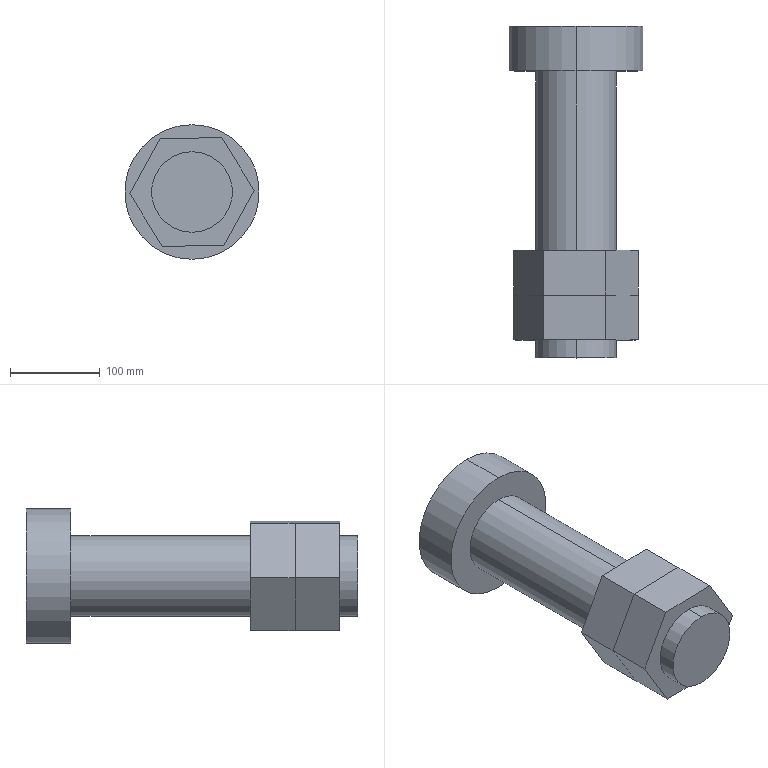Part | SolidWorks | features ICE 1, LPattern 1, Revolution 1 | 3 solids | 27 faces | box 150 x 370 x 150 mm | volume 3530229 mm3 | plane 19 | cylinder 8 | commonest cylinder face diameters 90 x6 150 x2
STEP:
#1=CARTESIAN_POINT('',(0.,345.893,-45.));
#2=VERTEX_POINT('',#1);
#3=CARTESIAN_POINT('',(0.,345.893,45.));
#4=VERTEX_POINT('',#3);
#5=CARTESIAN_POINT('',(0.,345.893,0.));
#6=DIRECTION('',(0.,-1.,0.));
#7=DIRECTION('',(0.,0.,-1.));
#8=AXIS2_PLACEMENT_3D('',#5,#6,#7);
#9=CIRCLE('',#8,45.);
#10=EDGE_CURVE('',#2,#4,#9,.T.);
#11=ORIENTED_EDGE('',*,*,#10,.T.);
#12=CARTESIAN_POINT('',(0.,25.893,45.));
#13=VERTEX_POINT('',#12);
#14=CARTESIAN_POINT('',(0.,0.,45.));
#15=DIRECTION('',(0.,-1.,0.));
#16=VECTOR('',#15,1000.);
#17=LINE('',#14,#16);
#18=EDGE_CURVE('',#4,#13,#17,.T.);
#19=ORIENTED_EDGE('',*,*,#18,.T.);
#20=CARTESIAN_POINT('',(0.,25.893,-45.));
#21=VERTEX_POINT('',#20);
#22=CARTESIAN_POINT('',(0.,25.893,0.));
#23=DIRECTION('',(0.,-1.,0.));
#24=DIRECTION('',(0.,0.,-1.));
#25=AXIS2_PLACEMENT_3D('',#22,#23,#24);
#26=CIRCLE('',#25,45.);
#27=EDGE_CURVE('',#21,#13,#26,.T.);
#28=ORIENTED_EDGE('',*,*,#27,.F.);
#29=CARTESIAN_POINT('',(0.,0.,-45.));
#30=DIRECTION('',(0.,-1.,0.));
#31=VECTOR('',#30,1000.);
#32=LINE('',#29,#31);
#33=EDGE_CURVE('',#2,#21,#32,.T.);
#34=ORIENTED_EDGE('',*,*,#33,.F.);
#35=EDGE_LOOP('',(#11,#19,#28,#34));
#36=FACE_OUTER_BOUND('',#35,.T.);
#37=CARTESIAN_POINT('',(0.,0.,0.));
#38=DIRECTION('',(0.,-1.,0.));
#39=DIRECTION('',(0.,0.,-1.));
#40=AXIS2_PLACEMENT_3D('',#37,#38,#39);
#41=CYLINDRICAL_SURFACE('',#40,45.);
#42=ADVANCED_FACE('',(#36),#41,.T.);
#43=CARTESIAN_POINT('',(0.,395.893,-75.));
#44=VERTEX_POINT('',#43);
#45=CARTESIAN_POINT('',(0.,395.893,75.));
#46=VERTEX_POINT('',#45);
#47=CARTESIAN_POINT('',(0.,395.893,0.));
#48=DIRECTION('',(0.,-1.,0.));
#49=DIRECTION('',(0.,0.,-1.));
#50=AXIS2_PLACEMENT_3D('',#47,#48,#49);
#51=CIRCLE('',#50,75.);
#52=EDGE_CURVE('',#44,#46,#51,.T.);
#53=ORIENTED_EDGE('',*,*,#52,.T.);
#54=CARTESIAN_POINT('',(0.,345.893,75.));
#55=VERTEX_POINT('',#54);
#56=CARTESIAN_POINT('',(0.,0.,75.));
#57=DIRECTION('',(0.,-1.,0.));
#58=VECTOR('',#57,1000.);
#59=LINE('',#56,#58);
#60=EDGE_CURVE('',#46,#55,#59,.T.);
#61=ORIENTED_EDGE('',*,*,#60,.T.);
#62=CARTESIAN_POINT('',(0.,345.893,-75.));
#63=VERTEX_POINT('',#62);
#64=CARTESIAN_POINT('',(0.,345.893,0.));
#65=DIRECTION('',(0.,-1.,0.));
#66=DIRECTION('',(0.,0.,-1.));
#67=AXIS2_PLACEMENT_3D('',#64,#65,#66);
#68=CIRCLE('',#67,75.);
#69=EDGE_CURVE('',#63,#55,#68,.T.);
#70=ORIENTED_EDGE('',*,*,#69,.F.);
#71=CARTESIAN_POINT('',(0.,0.,-75.));
#72=DIRECTION('',(0.,-1.,0.));
#73=VECTOR('',#72,1000.);
#74=LINE('',#71,#73);
#75=EDGE_CURVE('',#44,#63,#74,.T.);
#76=ORIENTED_EDGE('',*,*,#75,.F.);
#77=EDGE_LOOP('',(#53,#61,#70,#76));
#78=FACE_OUTER_BOUND('',#77,.T.);
#79=CARTESIAN_POINT('',(0.,0.,0.));
#80=DIRECTION('',(0.,-1.,0.));
#81=DIRECTION('',(0.,0.,-1.));
#82=AXIS2_PLACEMENT_3D('',#79,#80,#81);
#83=CYLINDRICAL_SURFACE('',#82,75.);
#84=ADVANCED_FACE('',(#78),#83,.T.);
#85=ORIENTED_EDGE('',*,*,#52,.F.);
#86=CARTESIAN_POINT('',(0.,395.893,0.));
#87=DIRECTION('',(0.,-1.,0.));
#88=DIRECTION('',(0.,0.,-1.));
#89=AXIS2_PLACEMENT_3D('',#86,#87,#88);
#90=CIRCLE('',#89,75.);
#91=EDGE_CURVE('',#46,#44,#90,.T.);
#92=ORIENTED_EDGE('',*,*,#91,.F.);
#93=EDGE_LOOP('',(#85,#92));
#94=FACE_OUTER_BOUND('',#93,.T.);
#95=CARTESIAN_POINT('',(0.,395.893,0.));
#96=DIRECTION('',(0.,1.,0.));
#97=DIRECTION('',(0.,0.,1.));
#98=AXIS2_PLACEMENT_3D('',#95,#96,#97);
#99=PLANE('',#98);
#100=ADVANCED_FACE('',(#94),#99,.T.);
#101=ORIENTED_EDGE('',*,*,#60,.F.);
#102=ORIENTED_EDGE('',*,*,#91,.T.);
#103=ORIENTED_EDGE('',*,*,#75,.T.);
#104=CARTESIAN_POINT('',(0.,345.893,0.));
#105=DIRECTION('',(0.,-1.,0.));
#106=DIRECTION('',(0.,0.,-1.));
#107=AXIS2_PLACEMENT_3D('',#104,#105,#106);
#108=CIRCLE('',#107,75.);
#109=EDGE_CURVE('',#55,#63,#108,.T.);
#110=ORIENTED_EDGE('',*,*,#109,.F.);
#111=EDGE_LOOP('',(#101,#102,#103,#110));
#112=FACE_OUTER_BOUND('',#111,.T.);
#113=CARTESIAN_POINT('',(0.,0.,0.));
#114=DIRECTION('',(0.,-1.,0.));
#115=DIRECTION('',(0.,0.,-1.));
#116=AXIS2_PLACEMENT_3D('',#113,#114,#115);
#117=CYLINDRICAL_SURFACE('',#116,75.);
#118=ADVANCED_FACE('',(#112),#117,.T.);
#119=ORIENTED_EDGE('',*,*,#69,.T.);
#120=ORIENTED_EDGE('',*,*,#109,.T.);
#121=EDGE_LOOP('',(#119,#120));
#122=FACE_OUTER_BOUND('',#121,.T.);
#123=ORIENTED_EDGE('',*,*,#10,.F.);
#124=CARTESIAN_POINT('',(0.,345.893,0.));
#125=DIRECTION('',(0.,-1.,0.));
#126=DIRECTION('',(0.,0.,-1.));
#127=AXIS2_PLACEMENT_3D('',#124,#125,#126);
#128=CIRCLE('',#127,45.);
#129=EDGE_CURVE('',#4,#2,#128,.T.);
#130=ORIENTED_EDGE('',*,*,#129,.F.);
#131=EDGE_LOOP('',(#123,#130));
#132=FACE_BOUND('',#131,.T.);
#133=CARTESIAN_POINT('',(75.,345.893,0.));
#134=DIRECTION('',(0.,-1.,0.));
#135=DIRECTION('',(0.,0.,-1.));
#136=AXIS2_PLACEMENT_3D('',#133,#134,#135);
#137=PLANE('',#136);
#138=ADVANCED_FACE('',(#122,#132),#137,.T.);
#139=ORIENTED_EDGE('',*,*,#18,.F.);
#140=ORIENTED_EDGE('',*,*,#129,.T.);
#141=ORIENTED_EDGE('',*,*,#33,.T.);
#142=CARTESIAN_POINT('',(0.,25.893,0.));
#143=DIRECTION('',(0.,-1.,0.));
#144=DIRECTION('',(0.,0.,-1.));
#145=AXIS2_PLACEMENT_3D('',#142,#143,#144);
#146=CIRCLE('',#145,45.);
#147=EDGE_CURVE('',#13,#21,#146,.T.);
#148=ORIENTED_EDGE('',*,*,#147,.F.);
#149=EDGE_LOOP('',(#139,#140,#141,#148));
#150=FACE_OUTER_BOUND('',#149,.T.);
#151=CARTESIAN_POINT('',(0.,0.,0.));
#152=DIRECTION('',(0.,-1.,0.));
#153=DIRECTION('',(0.,0.,-1.));
#154=AXIS2_PLACEMENT_3D('',#151,#152,#153);
#155=CYLINDRICAL_SURFACE('',#154,45.);
#156=ADVANCED_FACE('',(#150),#155,.T.);
#157=ORIENTED_EDGE('',*,*,#27,.T.);
#158=ORIENTED_EDGE('',*,*,#147,.T.);
#159=EDGE_LOOP('',(#157,#158));
#160=FACE_OUTER_BOUND('',#159,.T.);
#161=CARTESIAN_POINT('',(45.,25.893,0.));
#162=DIRECTION('',(0.,-1.,0.));
#163=DIRECTION('',(0.,0.,-1.));
#164=AXIS2_PLACEMENT_3D('',#161,#162,#163);
#165=PLANE('',#164);
#166=ADVANCED_FACE('',(#160),#165,.T.);
#167=CLOSED_SHELL('',(#42,#84,#100,#118,#138,#156,#166));
#168=MANIFOLD_SOLID_BREP('',#167);
#169=CARTESIAN_POINT('',(0.,95.893,45.));
#170=VERTEX_POINT('',#169);
#171=CARTESIAN_POINT('',(0.,95.893,-45.));
#172=VERTEX_POINT('',#171);
#173=CARTESIAN_POINT('',(0.,95.893,0.));
#174=DIRECTION('',(0.,-1.,0.));
#175=DIRECTION('',(0.,0.,-1.));
#176=AXIS2_PLACEMENT_3D('',#173,#174,#175);
#177=CIRCLE('',#176,45.);
#178=EDGE_CURVE('',#170,#172,#177,.T.);
#179=ORIENTED_EDGE('',*,*,#178,.T.);
#180=CARTESIAN_POINT('',(0.,145.893,-45.));
#181=VERTEX_POINT('',#180);
#182=CARTESIAN_POINT('',(0.,95.893,-45.));
#183=DIRECTION('',(0.,1.,0.));
#184=VECTOR('',#183,1000.);
#185=LINE('',#182,#184);
#186=EDGE_CURVE('',#172,#181,#185,.T.);
#187=ORIENTED_EDGE('',*,*,#186,.T.);
#188=CARTESIAN_POINT('',(0.,145.893,45.));
#189=VERTEX_POINT('',#188);
#190=CARTESIAN_POINT('',(0.,145.893,0.));
#191=DIRECTION('',(0.,-1.,0.));
#192=DIRECTION('',(0.,0.,-1.));
#193=AXIS2_PLACEMENT_3D('',#190,#191,#192);
#194=CIRCLE('',#193,45.);
#195=EDGE_CURVE('',#189,#181,#194,.T.);
#196=ORIENTED_EDGE('',*,*,#195,.F.);
#197=CARTESIAN_POINT('',(0.,95.893,45.));
#198=DIRECTION('',(0.,1.,0.));
#199=VECTOR('',#198,1000.);
#200=LINE('',#197,#199);
#201=EDGE_CURVE('',#170,#189,#200,.T.);
#202=ORIENTED_EDGE('',*,*,#201,.F.);
#203=EDGE_LOOP('',(#179,#187,#196,#202));
#204=FACE_OUTER_BOUND('',#203,.T.);
#205=CARTESIAN_POINT('',(0.,95.893,0.));
#206=DIRECTION('',(0.,1.,0.));
#207=DIRECTION('',(0.,0.,1.));
#208=AXIS2_PLACEMENT_3D('',#205,#206,#207);
#209=CYLINDRICAL_SURFACE('',#208,45.);
#210=ADVANCED_FACE('',(#204),#209,.F.);
#211=CARTESIAN_POINT('',(69.26,95.893,1.765));
#212=VERTEX_POINT('',#211);
#213=CARTESIAN_POINT('',(33.101,95.893,60.863));
#214=VERTEX_POINT('',#213);
#215=CARTESIAN_POINT('',(69.26,95.893,1.765));
#216=DIRECTION('',(-0.5219,0.,0.853));
#217=VECTOR('',#216,1000.);
#218=LINE('',#215,#217);
#219=EDGE_CURVE('',#212,#214,#218,.T.);
#220=ORIENTED_EDGE('',*,*,#219,.T.);
#221=CARTESIAN_POINT('',(-36.159,95.893,59.098));
#222=VERTEX_POINT('',#221);
#223=CARTESIAN_POINT('',(33.101,95.893,60.863));
#224=DIRECTION('',(-0.9997,0.,-0.02548));
#225=VECTOR('',#224,1000.);
#226=LINE('',#223,#225);
#227=EDGE_CURVE('',#214,#222,#226,.T.);
#228=ORIENTED_EDGE('',*,*,#227,.T.);
#229=CARTESIAN_POINT('',(-69.26,95.893,-1.765));
#230=VERTEX_POINT('',#229);
#231=CARTESIAN_POINT('',(-36.159,95.893,59.098));
#232=DIRECTION('',(-0.4778,0.,-0.8785));
#233=VECTOR('',#232,1000.);
#234=LINE('',#231,#233);
#235=EDGE_CURVE('',#222,#230,#234,.T.);
#236=ORIENTED_EDGE('',*,*,#235,.T.);
#237=CARTESIAN_POINT('',(-33.101,95.893,-60.863));
#238=VERTEX_POINT('',#237);
#239=CARTESIAN_POINT('',(-69.26,95.893,-1.765));
#240=DIRECTION('',(0.5219,0.,-0.853));
#241=VECTOR('',#240,1000.);
#242=LINE('',#239,#241);
#243=EDGE_CURVE('',#230,#238,#242,.T.);
#244=ORIENTED_EDGE('',*,*,#243,.T.);
#245=CARTESIAN_POINT('',(36.159,95.893,-59.098));
#246=VERTEX_POINT('',#245);
#247=CARTESIAN_POINT('',(-33.101,95.893,-60.863));
#248=DIRECTION('',(0.9997,0.,0.02548));
#249=VECTOR('',#248,1000.);
#250=LINE('',#247,#249);
#251=EDGE_CURVE('',#238,#246,#250,.T.);
#252=ORIENTED_EDGE('',*,*,#251,.T.);
#253=CARTESIAN_POINT('',(36.159,95.893,-59.098));
#254=DIRECTION('',(0.4778,0.,0.8785));
#255=VECTOR('',#254,1000.);
#256=LINE('',#253,#255);
#257=EDGE_CURVE('',#246,#212,#256,.T.);
#258=ORIENTED_EDGE('',*,*,#257,.T.);
#259=EDGE_LOOP('',(#220,#228,#236,#244,#252,#258));
#260=FACE_OUTER_BOUND('',#259,.T.);
#261=ORIENTED_EDGE('',*,*,#178,.F.);
#262=CARTESIAN_POINT('',(0.,95.893,0.));
#263=DIRECTION('',(0.,-1.,0.));
#264=DIRECTION('',(0.,0.,-1.));
#265=AXIS2_PLACEMENT_3D('',#262,#263,#264);
#266=CIRCLE('',#265,45.);
#267=EDGE_CURVE('',#172,#170,#266,.T.);
#268=ORIENTED_EDGE('',*,*,#267,.F.);
#269=EDGE_LOOP('',(#261,#268));
#270=FACE_BOUND('',#269,.T.);
#271=CARTESIAN_POINT('',(0.,95.893,0.));
#272=DIRECTION('',(0.,-1.,0.));
#273=DIRECTION('',(0.,0.,-1.));
#274=AXIS2_PLACEMENT_3D('',#271,#272,#273);
#275=PLANE('',#274);
#276=ADVANCED_FACE('',(#260,#270),#275,.T.);
#277=CARTESIAN_POINT('',(69.26,145.893,1.765));
#278=VERTEX_POINT('',#277);
#279=CARTESIAN_POINT('',(33.101,145.893,60.863));
#280=VERTEX_POINT('',#279);
#281=CARTESIAN_POINT('',(69.26,145.893,1.765));
#282=DIRECTION('',(-0.5219,0.,0.853));
#283=VECTOR('',#282,1000.);
#284=LINE('',#281,#283);
#285=EDGE_CURVE('',#278,#280,#284,.T.);
#286=ORIENTED_EDGE('',*,*,#285,.F.);
#287=CARTESIAN_POINT('',(36.159,145.893,-59.098));
#288=VERTEX_POINT('',#287);
#289=CARTESIAN_POINT('',(36.159,145.893,-59.098));
#290=DIRECTION('',(0.4778,0.,0.8785));
#291=VECTOR('',#290,1000.);
#292=LINE('',#289,#291);
#293=EDGE_CURVE('',#288,#278,#292,.T.);
#294=ORIENTED_EDGE('',*,*,#293,.F.);
#295=CARTESIAN_POINT('',(-33.101,145.893,-60.863));
#296=VERTEX_POINT('',#295);
#297=CARTESIAN_POINT('',(-33.101,145.893,-60.863));
#298=DIRECTION('',(0.9997,0.,0.02548));
#299=VECTOR('',#298,1000.);
#300=LINE('',#297,#299);
#301=EDGE_CURVE('',#296,#288,#300,.T.);
#302=ORIENTED_EDGE('',*,*,#301,.F.);
#303=CARTESIAN_POINT('',(-69.26,145.893,-1.765));
#304=VERTEX_POINT('',#303);
#305=CARTESIAN_POINT('',(-69.26,145.893,-1.765));
#306=DIRECTION('',(0.5219,0.,-0.853));
#307=VECTOR('',#306,1000.);
#308=LINE('',#305,#307);
#309=EDGE_CURVE('',#304,#296,#308,.T.);
#310=ORIENTED_EDGE('',*,*,#309,.F.);
#311=CARTESIAN_POINT('',(-36.159,145.893,59.098));
#312=VERTEX_POINT('',#311);
#313=CARTESIAN_POINT('',(-36.159,145.893,59.098));
#314=DIRECTION('',(-0.4778,0.,-0.8785));
#315=VECTOR('',#314,1000.);
#316=LINE('',#313,#315);
#317=EDGE_CURVE('',#312,#304,#316,.T.);
#318=ORIENTED_EDGE('',*,*,#317,.F.);
#319=CARTESIAN_POINT('',(33.101,145.893,60.863));
#320=DIRECTION('',(-0.9997,0.,-0.02548));
#321=VECTOR('',#320,1000.);
#322=LINE('',#319,#321);
#323=EDGE_CURVE('',#280,#312,#322,.T.);
#324=ORIENTED_EDGE('',*,*,#323,.F.);
#325=EDGE_LOOP('',(#286,#294,#302,#310,#318,#324));
#326=FACE_OUTER_BOUND('',#325,.T.);
#327=ORIENTED_EDGE('',*,*,#195,.T.);
#328=CARTESIAN_POINT('',(0.,145.893,0.));
#329=DIRECTION('',(0.,-1.,0.));
#330=DIRECTION('',(0.,0.,-1.));
#331=AXIS2_PLACEMENT_3D('',#328,#329,#330);
#332=CIRCLE('',#331,45.);
#333=EDGE_CURVE('',#181,#189,#332,.T.);
#334=ORIENTED_EDGE('',*,*,#333,.T.);
#335=EDGE_LOOP('',(#327,#334));
#336=FACE_BOUND('',#335,.T.);
#337=CARTESIAN_POINT('',(0.,145.893,0.));
#338=DIRECTION('',(0.,-1.,0.));
#339=DIRECTION('',(0.,0.,-1.));
#340=AXIS2_PLACEMENT_3D('',#337,#338,#339);
#341=PLANE('',#340);
#342=ADVANCED_FACE('',(#326,#336),#341,.F.);
#343=ORIENTED_EDGE('',*,*,#285,.T.);
#344=CARTESIAN_POINT('',(33.101,95.893,60.863));
#345=DIRECTION('',(0.,1.,0.));
#346=VECTOR('',#345,1000.);
#347=LINE('',#344,#346);
#348=EDGE_CURVE('',#214,#280,#347,.T.);
#349=ORIENTED_EDGE('',*,*,#348,.F.);
#350=ORIENTED_EDGE('',*,*,#219,.F.);
#351=CARTESIAN_POINT('',(69.26,95.893,1.765));
#352=DIRECTION('',(0.,1.,0.));
#353=VECTOR('',#352,1000.);
#354=LINE('',#351,#353);
#355=EDGE_CURVE('',#212,#278,#354,.T.);
#356=ORIENTED_EDGE('',*,*,#355,.T.);
#357=EDGE_LOOP('',(#343,#349,#350,#356));
#358=FACE_OUTER_BOUND('',#357,.T.);
#359=CARTESIAN_POINT('',(69.26,95.893,1.765));
#360=DIRECTION('',(-0.853,0.,-0.5219));
#361=DIRECTION('',(-0.5219,0.,0.853));
#362=AXIS2_PLACEMENT_3D('',#359,#360,#361);
#363=PLANE('',#362);
#364=ADVANCED_FACE('',(#358),#363,.F.);
#365=ORIENTED_EDGE('',*,*,#323,.T.);
#366=CARTESIAN_POINT('',(-36.159,95.893,59.098));
#367=DIRECTION('',(0.,1.,0.));
#368=VECTOR('',#367,1000.);
#369=LINE('',#366,#368);
#370=EDGE_CURVE('',#222,#312,#369,.T.);
#371=ORIENTED_EDGE('',*,*,#370,.F.);
#372=ORIENTED_EDGE('',*,*,#227,.F.);
#373=ORIENTED_EDGE('',*,*,#348,.T.);
#374=EDGE_LOOP('',(#365,#371,#372,#373));
#375=FACE_OUTER_BOUND('',#374,.T.);
#376=CARTESIAN_POINT('',(33.101,95.893,60.863));
#377=DIRECTION('',(0.02548,0.,-0.9997));
#378=DIRECTION('',(-0.9997,0.,-0.02548));
#379=AXIS2_PLACEMENT_3D('',#376,#377,#378);
#380=PLANE('',#379);
#381=ADVANCED_FACE('',(#375),#380,.F.);
#382=ORIENTED_EDGE('',*,*,#317,.T.);
#383=CARTESIAN_POINT('',(-69.26,95.893,-1.765));
#384=DIRECTION('',(0.,1.,0.));
#385=VECTOR('',#384,1000.);
#386=LINE('',#383,#385);
#387=EDGE_CURVE('',#230,#304,#386,.T.);
#388=ORIENTED_EDGE('',*,*,#387,.F.);
#389=ORIENTED_EDGE('',*,*,#235,.F.);
#390=ORIENTED_EDGE('',*,*,#370,.T.);
#391=EDGE_LOOP('',(#382,#388,#389,#390));
#392=FACE_OUTER_BOUND('',#391,.T.);
#393=CARTESIAN_POINT('',(-36.159,95.893,59.098));
#394=DIRECTION('',(0.8785,0.,-0.4778));
#395=DIRECTION('',(-0.4778,0.,-0.8785));
#396=AXIS2_PLACEMENT_3D('',#393,#394,#395);
#397=PLANE('',#396);
#398=ADVANCED_FACE('',(#392),#397,.F.);
#399=ORIENTED_EDGE('',*,*,#309,.T.);
#400=CARTESIAN_POINT('',(-33.101,95.893,-60.863));
#401=DIRECTION('',(0.,1.,0.));
#402=VECTOR('',#401,1000.);
#403=LINE('',#400,#402);
#404=EDGE_CURVE('',#238,#296,#403,.T.);
#405=ORIENTED_EDGE('',*,*,#404,.F.);
#406=ORIENTED_EDGE('',*,*,#243,.F.);
#407=ORIENTED_EDGE('',*,*,#387,.T.);
#408=EDGE_LOOP('',(#399,#405,#406,#407));
#409=FACE_OUTER_BOUND('',#408,.T.);
#410=CARTESIAN_POINT('',(-69.26,95.893,-1.765));
#411=DIRECTION('',(0.853,0.,0.5219));
#412=DIRECTION('',(0.5219,0.,-0.853));
#413=AXIS2_PLACEMENT_3D('',#410,#411,#412);
#414=PLANE('',#413);
#415=ADVANCED_FACE('',(#409),#414,.F.);
#416=ORIENTED_EDGE('',*,*,#301,.T.);
#417=CARTESIAN_POINT('',(36.159,95.893,-59.098));
#418=DIRECTION('',(0.,1.,0.));
#419=VECTOR('',#418,1000.);
#420=LINE('',#417,#419);
#421=EDGE_CURVE('',#246,#288,#420,.T.);
#422=ORIENTED_EDGE('',*,*,#421,.F.);
#423=ORIENTED_EDGE('',*,*,#251,.F.);
#424=ORIENTED_EDGE('',*,*,#404,.T.);
#425=EDGE_LOOP('',(#416,#422,#423,#424));
#426=FACE_OUTER_BOUND('',#425,.T.);
#427=CARTESIAN_POINT('',(-33.101,95.893,-60.863));
#428=DIRECTION('',(-0.02548,0.,0.9997));
#429=DIRECTION('',(0.9997,0.,0.02548));
#430=AXIS2_PLACEMENT_3D('',#427,#428,#429);
#431=PLANE('',#430);
#432=ADVANCED_FACE('',(#426),#431,.F.);
#433=ORIENTED_EDGE('',*,*,#293,.T.);
#434=ORIENTED_EDGE('',*,*,#355,.F.);
#435=ORIENTED_EDGE('',*,*,#257,.F.);
#436=ORIENTED_EDGE('',*,*,#421,.T.);
#437=EDGE_LOOP('',(#433,#434,#435,#436));
#438=FACE_OUTER_BOUND('',#437,.T.);
#439=CARTESIAN_POINT('',(36.159,95.893,-59.098));
#440=DIRECTION('',(-0.8785,0.,0.4778));
#441=DIRECTION('',(0.4778,0.,0.8785));
#442=AXIS2_PLACEMENT_3D('',#439,#440,#441);
#443=PLANE('',#442);
#444=ADVANCED_FACE('',(#438),#443,.F.);
#445=ORIENTED_EDGE('',*,*,#186,.F.);
#446=ORIENTED_EDGE('',*,*,#267,.T.);
#447=ORIENTED_EDGE('',*,*,#201,.T.);
#448=ORIENTED_EDGE('',*,*,#333,.F.);
#449=EDGE_LOOP('',(#445,#446,#447,#448));
#450=FACE_OUTER_BOUND('',#449,.T.);
#451=CARTESIAN_POINT('',(0.,95.893,0.));
#452=DIRECTION('',(0.,1.,0.));
#453=DIRECTION('',(0.,0.,1.));
#454=AXIS2_PLACEMENT_3D('',#451,#452,#453);
#455=CYLINDRICAL_SURFACE('',#454,45.);
#456=ADVANCED_FACE('',(#450),#455,.F.);
#457=CLOSED_SHELL('',(#210,#276,#342,#364,#381,#398,#415,#432,#444,#456));
#458=MANIFOLD_SOLID_BREP('',#457);
#459=CARTESIAN_POINT('',(0.,45.893,45.));
#460=VERTEX_POINT('',#459);
#461=CARTESIAN_POINT('',(0.,45.893,-45.));
#462=VERTEX_POINT('',#461);
#463=CARTESIAN_POINT('',(0.,45.893,0.));
#464=DIRECTION('',(0.,-1.,0.));
#465=DIRECTION('',(0.,0.,-1.));
#466=AXIS2_PLACEMENT_3D('',#463,#464,#465);
#467=CIRCLE('',#466,45.);
#468=EDGE_CURVE('',#460,#462,#467,.T.);
#469=ORIENTED_EDGE('',*,*,#468,.T.);
#470=CARTESIAN_POINT('',(0.,95.893,-45.));
#471=VERTEX_POINT('',#470);
#472=CARTESIAN_POINT('',(0.,45.893,-45.));
#473=DIRECTION('',(0.,1.,0.));
#474=VECTOR('',#473,1000.);
#475=LINE('',#472,#474);
#476=EDGE_CURVE('',#462,#471,#475,.T.);
#477=ORIENTED_EDGE('',*,*,#476,.T.);
#478=CARTESIAN_POINT('',(0.,95.893,45.));
#479=VERTEX_POINT('',#478);
#480=CARTESIAN_POINT('',(0.,95.893,0.));
#481=DIRECTION('',(0.,-1.,0.));
#482=DIRECTION('',(0.,0.,-1.));
#483=AXIS2_PLACEMENT_3D('',#480,#481,#482);
#484=CIRCLE('',#483,45.);
#485=EDGE_CURVE('',#479,#471,#484,.T.);
#486=ORIENTED_EDGE('',*,*,#485,.F.);
#487=CARTESIAN_POINT('',(0.,45.893,45.));
#488=DIRECTION('',(0.,1.,0.));
#489=VECTOR('',#488,1000.);
#490=LINE('',#487,#489);
#491=EDGE_CURVE('',#460,#479,#490,.T.);
#492=ORIENTED_EDGE('',*,*,#491,.F.);
#493=EDGE_LOOP('',(#469,#477,#486,#492));
#494=FACE_OUTER_BOUND('',#493,.T.);
#495=CARTESIAN_POINT('',(0.,45.893,0.));
#496=DIRECTION('',(0.,1.,0.));
#497=DIRECTION('',(0.,0.,1.));
#498=AXIS2_PLACEMENT_3D('',#495,#496,#497);
#499=CYLINDRICAL_SURFACE('',#498,45.);
#500=ADVANCED_FACE('',(#494),#499,.F.);
#501=CARTESIAN_POINT('',(69.26,45.893,1.765));
#502=VERTEX_POINT('',#501);
#503=CARTESIAN_POINT('',(33.101,45.893,60.863));
#504=VERTEX_POINT('',#503);
#505=CARTESIAN_POINT('',(69.26,45.893,1.765));
#506=DIRECTION('',(-0.5219,0.,0.853));
#507=VECTOR('',#506,1000.);
#508=LINE('',#505,#507);
#509=EDGE_CURVE('',#502,#504,#508,.T.);
#510=ORIENTED_EDGE('',*,*,#509,.T.);
#511=CARTESIAN_POINT('',(-36.159,45.893,59.098));
#512=VERTEX_POINT('',#511);
#513=CARTESIAN_POINT('',(33.101,45.893,60.863));
#514=DIRECTION('',(-0.9997,0.,-0.02548));
#515=VECTOR('',#514,1000.);
#516=LINE('',#513,#515);
#517=EDGE_CURVE('',#504,#512,#516,.T.);
#518=ORIENTED_EDGE('',*,*,#517,.T.);
#519=CARTESIAN_POINT('',(-69.26,45.893,-1.765));
#520=VERTEX_POINT('',#519);
#521=CARTESIAN_POINT('',(-36.159,45.893,59.098));
#522=DIRECTION('',(-0.4778,0.,-0.8785));
#523=VECTOR('',#522,1000.);
#524=LINE('',#521,#523);
#525=EDGE_CURVE('',#512,#520,#524,.T.);
#526=ORIENTED_EDGE('',*,*,#525,.T.);
#527=CARTESIAN_POINT('',(-33.101,45.893,-60.863));
#528=VERTEX_POINT('',#527);
#529=CARTESIAN_POINT('',(-69.26,45.893,-1.765));
#530=DIRECTION('',(0.5219,0.,-0.853));
#531=VECTOR('',#530,1000.);
#532=LINE('',#529,#531);
#533=EDGE_CURVE('',#520,#528,#532,.T.);
#534=ORIENTED_EDGE('',*,*,#533,.T.);
#535=CARTESIAN_POINT('',(36.159,45.893,-59.098));
#536=VERTEX_POINT('',#535);
#537=CARTESIAN_POINT('',(-33.101,45.893,-60.863));
#538=DIRECTION('',(0.9997,0.,0.02548));
#539=VECTOR('',#538,1000.);
#540=LINE('',#537,#539);
#541=EDGE_CURVE('',#528,#536,#540,.T.);
#542=ORIENTED_EDGE('',*,*,#541,.T.);
#543=CARTESIAN_POINT('',(36.159,45.893,-59.098));
#544=DIRECTION('',(0.4778,0.,0.8785));
#545=VECTOR('',#544,1000.);
#546=LINE('',#543,#545);
#547=EDGE_CURVE('',#536,#502,#546,.T.);
#548=ORIENTED_EDGE('',*,*,#547,.T.);
#549=EDGE_LOOP('',(#510,#518,#526,#534,#542,#548));
#550=FACE_OUTER_BOUND('',#549,.T.);
#551=ORIENTED_EDGE('',*,*,#468,.F.);
#552=CARTESIAN_POINT('',(0.,45.893,0.));
#553=DIRECTION('',(0.,-1.,0.));
#554=DIRECTION('',(0.,0.,-1.));
#555=AXIS2_PLACEMENT_3D('',#552,#553,#554);
#556=CIRCLE('',#555,45.);
#557=EDGE_CURVE('',#462,#460,#556,.T.);
#558=ORIENTED_EDGE('',*,*,#557,.F.);
#559=EDGE_LOOP('',(#551,#558));
#560=FACE_BOUND('',#559,.T.);
#561=CARTESIAN_POINT('',(0.,45.893,0.));
#562=DIRECTION('',(0.,-1.,0.));
#563=DIRECTION('',(0.,0.,-1.));
#564=AXIS2_PLACEMENT_3D('',#561,#562,#563);
#565=PLANE('',#564);
#566=ADVANCED_FACE('',(#550,#560),#565,.T.);
#567=CARTESIAN_POINT('',(69.26,95.893,1.765));
#568=VERTEX_POINT('',#567);
#569=CARTESIAN_POINT('',(33.101,95.893,60.863));
#570=VERTEX_POINT('',#569);
#571=CARTESIAN_POINT('',(69.26,95.893,1.765));
#572=DIRECTION('',(-0.5219,0.,0.853));
#573=VECTOR('',#572,1000.);
#574=LINE('',#571,#573);
#575=EDGE_CURVE('',#568,#570,#574,.T.);
#576=ORIENTED_EDGE('',*,*,#575,.F.);
#577=CARTESIAN_POINT('',(36.159,95.893,-59.098));
#578=VERTEX_POINT('',#577);
#579=CARTESIAN_POINT('',(36.159,95.893,-59.098));
#580=DIRECTION('',(0.4778,0.,0.8785));
#581=VECTOR('',#580,1000.);
#582=LINE('',#579,#581);
#583=EDGE_CURVE('',#578,#568,#582,.T.);
#584=ORIENTED_EDGE('',*,*,#583,.F.);
#585=CARTESIAN_POINT('',(-33.101,95.893,-60.863));
#586=VERTEX_POINT('',#585);
#587=CARTESIAN_POINT('',(-33.101,95.893,-60.863));
#588=DIRECTION('',(0.9997,0.,0.02548));
#589=VECTOR('',#588,1000.);
#590=LINE('',#587,#589);
#591=EDGE_CURVE('',#586,#578,#590,.T.);
#592=ORIENTED_EDGE('',*,*,#591,.F.);
#593=CARTESIAN_POINT('',(-69.26,95.893,-1.765));
#594=VERTEX_POINT('',#593);
#595=CARTESIAN_POINT('',(-69.26,95.893,-1.765));
#596=DIRECTION('',(0.5219,0.,-0.853));
#597=VECTOR('',#596,1000.);
#598=LINE('',#595,#597);
#599=EDGE_CURVE('',#594,#586,#598,.T.);
#600=ORIENTED_EDGE('',*,*,#599,.F.);
#601=CARTESIAN_POINT('',(-36.159,95.893,59.098));
#602=VERTEX_POINT('',#601);
#603=CARTESIAN_POINT('',(-36.159,95.893,59.098));
#604=DIRECTION('',(-0.4778,0.,-0.8785));
#605=VECTOR('',#604,1000.);
#606=LINE('',#603,#605);
#607=EDGE_CURVE('',#602,#594,#606,.T.);
#608=ORIENTED_EDGE('',*,*,#607,.F.);
#609=CARTESIAN_POINT('',(33.101,95.893,60.863));
#610=DIRECTION('',(-0.9997,0.,-0.02548));
#611=VECTOR('',#610,1000.);
#612=LINE('',#609,#611);
#613=EDGE_CURVE('',#570,#602,#612,.T.);
#614=ORIENTED_EDGE('',*,*,#613,.F.);
#615=EDGE_LOOP('',(#576,#584,#592,#600,#608,#614));
#616=FACE_OUTER_BOUND('',#615,.T.);
#617=ORIENTED_EDGE('',*,*,#485,.T.);
#618=CARTESIAN_POINT('',(0.,95.893,0.));
#619=DIRECTION('',(0.,-1.,0.));
#620=DIRECTION('',(0.,0.,-1.));
#621=AXIS2_PLACEMENT_3D('',#618,#619,#620);
#622=CIRCLE('',#621,45.);
#623=EDGE_CURVE('',#471,#479,#622,.T.);
#624=ORIENTED_EDGE('',*,*,#623,.T.);
#625=EDGE_LOOP('',(#617,#624));
#626=FACE_BOUND('',#625,.T.);
#627=CARTESIAN_POINT('',(0.,95.893,0.));
#628=DIRECTION('',(0.,-1.,0.));
#629=DIRECTION('',(0.,0.,-1.));
#630=AXIS2_PLACEMENT_3D('',#627,#628,#629);
#631=PLANE('',#630);
#632=ADVANCED_FACE('',(#616,#626),#631,.F.);
#633=ORIENTED_EDGE('',*,*,#575,.T.);
#634=CARTESIAN_POINT('',(33.101,45.893,60.863));
#635=DIRECTION('',(0.,1.,0.));
#636=VECTOR('',#635,1000.);
#637=LINE('',#634,#636);
#638=EDGE_CURVE('',#504,#570,#637,.T.);
#639=ORIENTED_EDGE('',*,*,#638,.F.);
#640=ORIENTED_EDGE('',*,*,#509,.F.);
#641=CARTESIAN_POINT('',(69.26,45.893,1.765));
#642=DIRECTION('',(0.,1.,0.));
#643=VECTOR('',#642,1000.);
#644=LINE('',#641,#643);
#645=EDGE_CURVE('',#502,#568,#644,.T.);
#646=ORIENTED_EDGE('',*,*,#645,.T.);
#647=EDGE_LOOP('',(#633,#639,#640,#646));
#648=FACE_OUTER_BOUND('',#647,.T.);
#649=CARTESIAN_POINT('',(69.26,45.893,1.765));
#650=DIRECTION('',(-0.853,0.,-0.5219));
#651=DIRECTION('',(-0.5219,0.,0.853));
#652=AXIS2_PLACEMENT_3D('',#649,#650,#651);
#653=PLANE('',#652);
#654=ADVANCED_FACE('',(#648),#653,.F.);
#655=ORIENTED_EDGE('',*,*,#613,.T.);
#656=CARTESIAN_POINT('',(-36.159,45.893,59.098));
#657=DIRECTION('',(0.,1.,0.));
#658=VECTOR('',#657,1000.);
#659=LINE('',#656,#658);
#660=EDGE_CURVE('',#512,#602,#659,.T.);
#661=ORIENTED_EDGE('',*,*,#660,.F.);
#662=ORIENTED_EDGE('',*,*,#517,.F.);
#663=ORIENTED_EDGE('',*,*,#638,.T.);
#664=EDGE_LOOP('',(#655,#661,#662,#663));
#665=FACE_OUTER_BOUND('',#664,.T.);
#666=CARTESIAN_POINT('',(33.101,45.893,60.863));
#667=DIRECTION('',(0.02548,0.,-0.9997));
#668=DIRECTION('',(-0.9997,0.,-0.02548));
#669=AXIS2_PLACEMENT_3D('',#666,#667,#668);
#670=PLANE('',#669);
#671=ADVANCED_FACE('',(#665),#670,.F.);
#672=ORIENTED_EDGE('',*,*,#607,.T.);
#673=CARTESIAN_POINT('',(-69.26,45.893,-1.765));
#674=DIRECTION('',(0.,1.,0.));
#675=VECTOR('',#674,1000.);
#676=LINE('',#673,#675);
#677=EDGE_CURVE('',#520,#594,#676,.T.);
#678=ORIENTED_EDGE('',*,*,#677,.F.);
#679=ORIENTED_EDGE('',*,*,#525,.F.);
#680=ORIENTED_EDGE('',*,*,#660,.T.);
#681=EDGE_LOOP('',(#672,#678,#679,#680));
#682=FACE_OUTER_BOUND('',#681,.T.);
#683=CARTESIAN_POINT('',(-36.159,45.893,59.098));
#684=DIRECTION('',(0.8785,0.,-0.4778));
#685=DIRECTION('',(-0.4778,0.,-0.8785));
#686=AXIS2_PLACEMENT_3D('',#683,#684,#685);
#687=PLANE('',#686);
#688=ADVANCED_FACE('',(#682),#687,.F.);
#689=ORIENTED_EDGE('',*,*,#599,.T.);
#690=CARTESIAN_POINT('',(-33.101,45.893,-60.863));
#691=DIRECTION('',(0.,1.,0.));
#692=VECTOR('',#691,1000.);
#693=LINE('',#690,#692);
#694=EDGE_CURVE('',#528,#586,#693,.T.);
#695=ORIENTED_EDGE('',*,*,#694,.F.);
#696=ORIENTED_EDGE('',*,*,#533,.F.);
#697=ORIENTED_EDGE('',*,*,#677,.T.);
#698=EDGE_LOOP('',(#689,#695,#696,#697));
#699=FACE_OUTER_BOUND('',#698,.T.);
#700=CARTESIAN_POINT('',(-69.26,45.893,-1.765));
#701=DIRECTION('',(0.853,0.,0.5219));
#702=DIRECTION('',(0.5219,0.,-0.853));
#703=AXIS2_PLACEMENT_3D('',#700,#701,#702);
#704=PLANE('',#703);
#705=ADVANCED_FACE('',(#699),#704,.F.);
#706=ORIENTED_EDGE('',*,*,#591,.T.);
#707=CARTESIAN_POINT('',(36.159,45.893,-59.098));
#708=DIRECTION('',(0.,1.,0.));
#709=VECTOR('',#708,1000.);
#710=LINE('',#707,#709);
#711=EDGE_CURVE('',#536,#578,#710,.T.);
#712=ORIENTED_EDGE('',*,*,#711,.F.);
#713=ORIENTED_EDGE('',*,*,#541,.F.);
#714=ORIENTED_EDGE('',*,*,#694,.T.);
#715=EDGE_LOOP('',(#706,#712,#713,#714));
#716=FACE_OUTER_BOUND('',#715,.T.);
#717=CARTESIAN_POINT('',(-33.101,45.893,-60.863));
#718=DIRECTION('',(-0.02548,0.,0.9997));
#719=DIRECTION('',(0.9997,0.,0.02548));
#720=AXIS2_PLACEMENT_3D('',#717,#718,#719);
#721=PLANE('',#720);
#722=ADVANCED_FACE('',(#716),#721,.F.);
#723=ORIENTED_EDGE('',*,*,#583,.T.);
#724=ORIENTED_EDGE('',*,*,#645,.F.);
#725=ORIENTED_EDGE('',*,*,#547,.F.);
#726=ORIENTED_EDGE('',*,*,#711,.T.);
#727=EDGE_LOOP('',(#723,#724,#725,#726));
#728=FACE_OUTER_BOUND('',#727,.T.);
#729=CARTESIAN_POINT('',(36.159,45.893,-59.098));
#730=DIRECTION('',(-0.8785,0.,0.4778));
#731=DIRECTION('',(0.4778,0.,0.8785));
#732=AXIS2_PLACEMENT_3D('',#729,#730,#731);
#733=PLANE('',#732);
#734=ADVANCED_FACE('',(#728),#733,.F.);
#735=ORIENTED_EDGE('',*,*,#476,.F.);
#736=ORIENTED_EDGE('',*,*,#557,.T.);
#737=ORIENTED_EDGE('',*,*,#491,.T.);
#738=ORIENTED_EDGE('',*,*,#623,.F.);
#739=EDGE_LOOP('',(#735,#736,#737,#738));
#740=FACE_OUTER_BOUND('',#739,.T.);
#741=CARTESIAN_POINT('',(0.,45.893,0.));
#742=DIRECTION('',(0.,1.,0.));
#743=DIRECTION('',(0.,0.,1.));
#744=AXIS2_PLACEMENT_3D('',#741,#742,#743);
#745=CYLINDRICAL_SURFACE('',#744,45.);
#746=ADVANCED_FACE('',(#740),#745,.F.);
#747=CLOSED_SHELL('',(#500,#566,#632,#654,#671,#688,#705,#722,#734,#746));
#748=MANIFOLD_SOLID_BREP('',#747);
#749=CARTESIAN_POINT('',(0.,0.,0.));
#750=DIRECTION('',(0.,0.,1.));
#751=DIRECTION('',(1.,0.,0.));
#752=AXIS2_PLACEMENT_3D('',#749,#750,#751);
#753=(LENGTH_UNIT()NAMED_UNIT(*)SI_UNIT(.MILLI.,.METRE.));
#754=UNCERTAINTY_MEASURE_WITH_UNIT(LENGTH_MEASURE(0.00001),#753,'','');
#755=(NAMED_UNIT(*)PLANE_ANGLE_UNIT()SI_UNIT($,.RADIAN.));
#756=(NAMED_UNIT(*)SI_UNIT($,.STERADIAN.)SOLID_ANGLE_UNIT());
#757=(GEOMETRIC_REPRESENTATION_CONTEXT(3)GLOBAL_UNCERTAINTY_ASSIGNED_CONTEXT((#754))GLOBAL_UNIT_ASSIGNED_CONTEXT((#753,#755,#756))REPRESENTATION_CONTEXT('',''));
#758=ADVANCED_BREP_SHAPE_REPRESENTATION('',(#168,#458,#748,#752),#757);